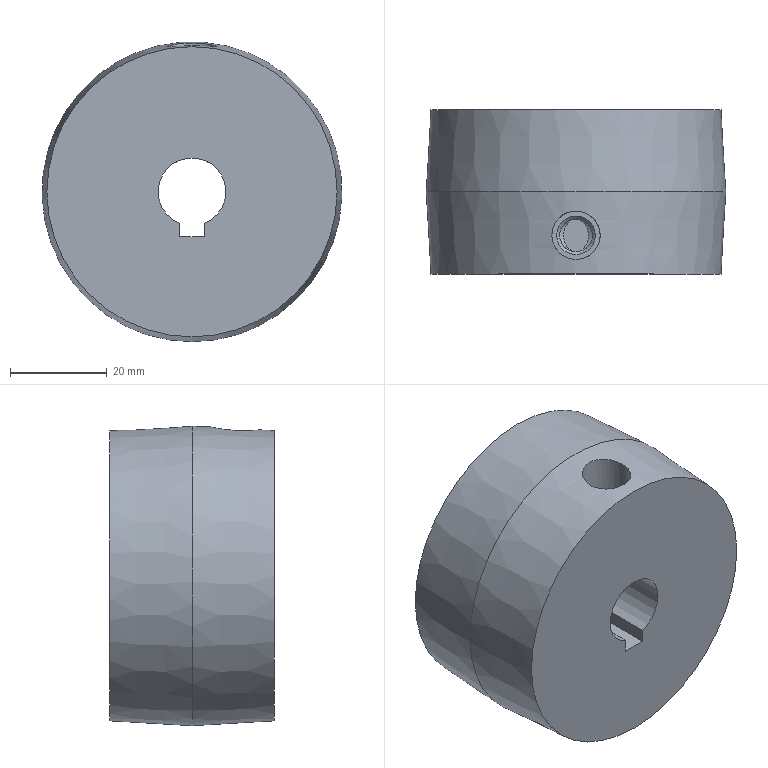Part | NX | features DATUM_CSYS 6, SKETCH 5, HOLE PACKAGE 2, SIMPLE HOLE 2, SWP104 2, EXTRUDE 1, SYMBOLIC_THREAD 1 | 1 solid | 16 faces | box 62 x 34 x 62 mm | volume 57319 mm3 | plane 7 | cone 5 | cylinder 4 | commonest cylinder face diameters 6.8 x1 10 x1 14 x1 52 x1
STEP:
#1=CARTESIAN_POINT('',(0.,0.,-30.));
#2=VERTEX_POINT('',#1);
#3=CARTESIAN_POINT('',(0.,0.,0.));
#4=DIRECTION('',(0.,-1.,0.));
#5=DIRECTION('',(0.,0.,-1.));
#6=AXIS2_PLACEMENT_3D('',#3,#4,#5);
#7=CIRCLE('',#6,30.);
#8=EDGE_CURVE('',#2,#2,#7,.T.);
#9=ORIENTED_EDGE('',*,*,#8,.F.);
#10=EDGE_LOOP('',(#9));
#11=FACE_BOUND('',#10,.T.);
#12=CARTESIAN_POINT('',(0.,17.,-31.));
#13=VERTEX_POINT('',#12);
#14=CARTESIAN_POINT('',(0.,17.,0.));
#15=DIRECTION('',(0.,-1.,0.));
#16=DIRECTION('',(0.,0.,-1.));
#17=AXIS2_PLACEMENT_3D('',#14,#15,#16);
#18=CIRCLE('',#17,31.);
#19=EDGE_CURVE('',#13,#13,#18,.T.);
#20=ORIENTED_EDGE('',*,*,#19,.T.);
#21=EDGE_LOOP('',(#20));
#22=FACE_BOUND('',#21,.T.);
#23=CARTESIAN_POINT('',(-3.572,4.502,30.053));
#24=VERTEX_POINT('',#23);
#25=CARTESIAN_POINT('',(-5.539,8.08,29.959));
#26=CARTESIAN_POINT('',(-3.962,4.118,30.028));
#27=CARTESIAN_POINT('',(-0.0481,2.459,30.249));
#28=CARTESIAN_POINT('',(3.888,4.047,30.035));
#29=CARTESIAN_POINT('',(5.541,7.972,29.952));
#30=CARTESIAN_POINT('',(3.949,11.879,30.491));
#31=CARTESIAN_POINT('',(0.05764,13.542,30.898));
#32=CARTESIAN_POINT('',(-3.879,11.952,30.507));
#33=CARTESIAN_POINT('',(-5.539,8.08,29.959));
#34=CARTESIAN_POINT('',(-3.962,4.118,30.028));
#35=CARTESIAN_POINT('',(-0.0481,2.459,30.249));
#36=B_SPLINE_CURVE_WITH_KNOTS('',3,(#25,#26,#27,#28,#29,#30,#31,#32,#33,#34,#35),.UNSPECIFIED.,.T.,.F.,(1,1,1,1,1,1,1,1,1,1,1,1,1,1,1),(-0.01175,-0.007835,-0.003918,0.,0.003918,0.007835,0.01175,0.01567,0.01959,0.02351,0.02742,0.03134,0.03526,0.03918,0.04309),.UNSPECIFIED.);
#37=EDGE_CURVE('',#24,#24,#36,.T.);
#38=ORIENTED_EDGE('',*,*,#37,.F.);
#39=EDGE_LOOP('',(#38));
#40=FACE_BOUND('',#39,.T.);
#41=CARTESIAN_POINT('',(0.,17.,0.));
#42=DIRECTION('',(0.,1.,0.));
#43=DIRECTION('',(0.,0.,1.));
#44=AXIS2_PLACEMENT_3D('',#41,#42,#43);
#45=CONICAL_SURFACE('',#44,31.,0.05876);
#46=ADVANCED_FACE('',(#11,#22,#40),#45,.T.);
#47=CARTESIAN_POINT('',(0.,16.,-26.));
#48=VERTEX_POINT('',#47);
#49=CARTESIAN_POINT('',(0.,16.,0.));
#50=DIRECTION('',(0.,-1.,0.));
#51=DIRECTION('',(0.,0.,-1.));
#52=AXIS2_PLACEMENT_3D('',#49,#50,#51);
#53=CIRCLE('',#52,26.);
#54=EDGE_CURVE('',#48,#48,#53,.F.);
#55=ORIENTED_EDGE('',*,*,#54,.T.);
#56=EDGE_LOOP('',(#55));
#57=FACE_BOUND('',#56,.T.);
#58=CARTESIAN_POINT('',(2.5,16.,-9.3));
#59=VERTEX_POINT('',#58);
#60=CARTESIAN_POINT('',(-2.5,16.,-9.3));
#61=VERTEX_POINT('',#60);
#62=CARTESIAN_POINT('',(-2.5,16.,-9.3));
#63=DIRECTION('',(-1.,0.,0.));
#64=VECTOR('',#63,1000.);
#65=LINE('',#62,#64);
#66=EDGE_CURVE('',#59,#61,#65,.T.);
#67=ORIENTED_EDGE('',*,*,#66,.F.);
#68=CARTESIAN_POINT('',(2.5,16.,-6.538));
#69=VERTEX_POINT('',#68);
#70=CARTESIAN_POINT('',(2.5,16.,-9.3));
#71=DIRECTION('',(0.,0.,-1.));
#72=VECTOR('',#71,1000.);
#73=LINE('',#70,#72);
#74=EDGE_CURVE('',#69,#59,#73,.T.);
#75=ORIENTED_EDGE('',*,*,#74,.F.);
#76=CARTESIAN_POINT('',(-2.5,16.,-6.538));
#77=VERTEX_POINT('',#76);
#78=CARTESIAN_POINT('',(0.,16.,0.));
#79=DIRECTION('',(0.,-1.,0.));
#80=DIRECTION('',(0.,0.,-1.));
#81=AXIS2_PLACEMENT_3D('',#78,#79,#80);
#82=CIRCLE('',#81,7.);
#83=EDGE_CURVE('',#77,#69,#82,.F.);
#84=ORIENTED_EDGE('',*,*,#83,.F.);
#85=CARTESIAN_POINT('',(-2.5,16.,-6.538));
#86=DIRECTION('',(0.,0.,1.));
#87=VECTOR('',#86,1000.);
#88=LINE('',#85,#87);
#89=EDGE_CURVE('',#61,#77,#88,.T.);
#90=ORIENTED_EDGE('',*,*,#89,.F.);
#91=EDGE_LOOP('',(#67,#75,#84,#90));
#92=FACE_BOUND('',#91,.T.);
#93=CARTESIAN_POINT('',(0.,16.,0.));
#94=DIRECTION('',(0.,-1.,0.));
#95=DIRECTION('',(0.,0.,-1.));
#96=AXIS2_PLACEMENT_3D('',#93,#94,#95);
#97=PLANE('',#96);
#98=ADVANCED_FACE('',(#57,#92),#97,.F.);
#99=CARTESIAN_POINT('',(2.5,0.,-9.3));
#100=VERTEX_POINT('',#99);
#101=CARTESIAN_POINT('',(2.5,0.,-6.538));
#102=VERTEX_POINT('',#101);
#103=CARTESIAN_POINT('',(2.5,0.,-9.3));
#104=DIRECTION('',(0.,0.,1.));
#105=VECTOR('',#104,1000.);
#106=LINE('',#103,#105);
#107=EDGE_CURVE('',#100,#102,#106,.T.);
#108=ORIENTED_EDGE('',*,*,#107,.F.);
#109=CARTESIAN_POINT('',(-2.5,0.,-9.3));
#110=VERTEX_POINT('',#109);
#111=CARTESIAN_POINT('',(-2.5,0.,-9.3));
#112=DIRECTION('',(1.,0.,0.));
#113=VECTOR('',#112,1000.);
#114=LINE('',#111,#113);
#115=EDGE_CURVE('',#110,#100,#114,.T.);
#116=ORIENTED_EDGE('',*,*,#115,.F.);
#117=CARTESIAN_POINT('',(-2.5,0.,-6.538));
#118=VERTEX_POINT('',#117);
#119=CARTESIAN_POINT('',(-2.5,0.,-6.538));
#120=DIRECTION('',(0.,0.,-1.));
#121=VECTOR('',#120,1000.);
#122=LINE('',#119,#121);
#123=EDGE_CURVE('',#118,#110,#122,.T.);
#124=ORIENTED_EDGE('',*,*,#123,.F.);
#125=CARTESIAN_POINT('',(0.,0.,0.));
#126=DIRECTION('',(0.,-1.,0.));
#127=DIRECTION('',(1.,0.,0.));
#128=AXIS2_PLACEMENT_3D('',#125,#126,#127);
#129=CIRCLE('',#128,7.);
#130=EDGE_CURVE('',#102,#118,#129,.T.);
#131=ORIENTED_EDGE('',*,*,#130,.F.);
#132=EDGE_LOOP('',(#108,#116,#124,#131));
#133=FACE_BOUND('',#132,.T.);
#134=ORIENTED_EDGE('',*,*,#8,.T.);
#135=EDGE_LOOP('',(#134));
#136=FACE_BOUND('',#135,.T.);
#137=CARTESIAN_POINT('',(0.,0.,30.));
#138=DIRECTION('',(0.,1.,0.));
#139=DIRECTION('',(0.,0.,1.));
#140=AXIS2_PLACEMENT_3D('',#137,#138,#139);
#141=PLANE('',#140);
#142=ADVANCED_FACE('',(#133,#136),#141,.F.);
#143=CARTESIAN_POINT('',(0.,34.,-26.));
#144=VERTEX_POINT('',#143);
#145=CARTESIAN_POINT('',(0.,34.,0.));
#146=DIRECTION('',(0.,-1.,0.));
#147=DIRECTION('',(0.,0.,-1.));
#148=AXIS2_PLACEMENT_3D('',#145,#146,#147);
#149=CIRCLE('',#148,26.);
#150=EDGE_CURVE('',#144,#144,#149,.T.);
#151=ORIENTED_EDGE('',*,*,#150,.T.);
#152=EDGE_LOOP('',(#151));
#153=FACE_BOUND('',#152,.T.);
#154=CARTESIAN_POINT('',(0.,34.,-30.));
#155=VERTEX_POINT('',#154);
#156=CARTESIAN_POINT('',(0.,34.,0.));
#157=DIRECTION('',(0.,-1.,0.));
#158=DIRECTION('',(0.,0.,-1.));
#159=AXIS2_PLACEMENT_3D('',#156,#157,#158);
#160=CIRCLE('',#159,30.);
#161=EDGE_CURVE('',#155,#155,#160,.T.);
#162=ORIENTED_EDGE('',*,*,#161,.F.);
#163=EDGE_LOOP('',(#162));
#164=FACE_BOUND('',#163,.T.);
#165=CARTESIAN_POINT('',(0.,34.,0.));
#166=DIRECTION('',(0.,-1.,0.));
#167=DIRECTION('',(0.,0.,-1.));
#168=AXIS2_PLACEMENT_3D('',#165,#166,#167);
#169=PLANE('',#168);
#170=ADVANCED_FACE('',(#153,#164),#169,.F.);
#171=ORIENTED_EDGE('',*,*,#19,.F.);
#172=EDGE_LOOP('',(#171));
#173=FACE_BOUND('',#172,.T.);
#174=ORIENTED_EDGE('',*,*,#161,.T.);
#175=EDGE_LOOP('',(#174));
#176=FACE_BOUND('',#175,.T.);
#177=CARTESIAN_POINT('',(0.,34.,0.));
#178=DIRECTION('',(0.,-1.,0.));
#179=DIRECTION('',(0.,0.,-1.));
#180=AXIS2_PLACEMENT_3D('',#177,#178,#179);
#181=CONICAL_SURFACE('',#180,30.,0.05876);
#182=ADVANCED_FACE('',(#173,#176),#181,.T.);
#183=ORIENTED_EDGE('',*,*,#54,.F.);
#184=EDGE_LOOP('',(#183));
#185=FACE_BOUND('',#184,.T.);
#186=ORIENTED_EDGE('',*,*,#150,.F.);
#187=EDGE_LOOP('',(#186));
#188=FACE_BOUND('',#187,.T.);
#189=CARTESIAN_POINT('',(0.,34.,0.));
#190=DIRECTION('',(0.,-1.,0.));
#191=DIRECTION('',(0.,0.,-1.));
#192=AXIS2_PLACEMENT_3D('',#189,#190,#191);
#193=CYLINDRICAL_SURFACE('',#192,26.);
#194=ADVANCED_FACE('',(#185,#188),#193,.F.);
#195=ORIENTED_EDGE('',*,*,#66,.T.);
#196=CARTESIAN_POINT('',(-2.5,55000.,-9.3));
#197=DIRECTION('',(0.,-1.,0.));
#198=VECTOR('',#197,1000.);
#199=LINE('',#196,#198);
#200=EDGE_CURVE('',#110,#61,#199,.F.);
#201=ORIENTED_EDGE('',*,*,#200,.F.);
#202=ORIENTED_EDGE('',*,*,#115,.T.);
#203=CARTESIAN_POINT('',(2.5,55000.,-9.3));
#204=DIRECTION('',(0.,-1.,0.));
#205=VECTOR('',#204,1000.);
#206=LINE('',#203,#205);
#207=EDGE_CURVE('',#100,#59,#206,.F.);
#208=ORIENTED_EDGE('',*,*,#207,.T.);
#209=EDGE_LOOP('',(#195,#201,#202,#208));
#210=FACE_BOUND('',#209,.T.);
#211=CARTESIAN_POINT('',(-2.5,55000.,-9.3));
#212=DIRECTION('',(0.,0.,-1.));
#213=DIRECTION('',(-1.,0.,0.));
#214=AXIS2_PLACEMENT_3D('',#211,#212,#213);
#215=PLANE('',#214);
#216=ADVANCED_FACE('',(#210),#215,.F.);
#217=ORIENTED_EDGE('',*,*,#74,.T.);
#218=ORIENTED_EDGE('',*,*,#207,.F.);
#219=ORIENTED_EDGE('',*,*,#107,.T.);
#220=CARTESIAN_POINT('',(2.5,55000.,-6.538));
#221=DIRECTION('',(0.,-1.,0.));
#222=VECTOR('',#221,1000.);
#223=LINE('',#220,#222);
#224=EDGE_CURVE('',#102,#69,#223,.F.);
#225=ORIENTED_EDGE('',*,*,#224,.T.);
#226=EDGE_LOOP('',(#217,#218,#219,#225));
#227=FACE_BOUND('',#226,.T.);
#228=CARTESIAN_POINT('',(2.5,55000.,-9.3));
#229=DIRECTION('',(1.,0.,0.));
#230=DIRECTION('',(0.,0.,-1.));
#231=AXIS2_PLACEMENT_3D('',#228,#229,#230);
#232=PLANE('',#231);
#233=ADVANCED_FACE('',(#227),#232,.F.);
#234=ORIENTED_EDGE('',*,*,#89,.T.);
#235=CARTESIAN_POINT('',(-2.5,55000.,-6.538));
#236=DIRECTION('',(0.,-1.,0.));
#237=VECTOR('',#236,1000.);
#238=LINE('',#235,#237);
#239=EDGE_CURVE('',#118,#77,#238,.F.);
#240=ORIENTED_EDGE('',*,*,#239,.F.);
#241=ORIENTED_EDGE('',*,*,#123,.T.);
#242=ORIENTED_EDGE('',*,*,#200,.T.);
#243=EDGE_LOOP('',(#234,#240,#241,#242));
#244=FACE_BOUND('',#243,.T.);
#245=CARTESIAN_POINT('',(-2.5,55000.,-6.538));
#246=DIRECTION('',(-1.,0.,0.));
#247=DIRECTION('',(0.,0.,1.));
#248=AXIS2_PLACEMENT_3D('',#245,#246,#247);
#249=PLANE('',#248);
#250=ADVANCED_FACE('',(#244),#249,.F.);
#251=CARTESIAN_POINT('',(0.,11.4,7.));
#252=VERTEX_POINT('',#251);
#253=CARTESIAN_POINT('',(0.,4.6,7.));
#254=VERTEX_POINT('',#253);
#255=CARTESIAN_POINT('',(0.,11.4,7.));
#256=CARTESIAN_POINT('',(-0.7926,11.4,7.));
#257=CARTESIAN_POINT('',(-2.181,10.356,6.702));
#258=CARTESIAN_POINT('',(-2.78,7.997,6.41));
#259=CARTESIAN_POINT('',(-2.178,5.641,6.703));
#260=CARTESIAN_POINT('',(-0.7919,4.6,7.));
#261=CARTESIAN_POINT('',(0.,4.6,7.));
#262=B_SPLINE_CURVE_WITH_KNOTS('',3,(#255,#256,#257,#258,#259,#260,#261),.UNSPECIFIED.,.F.,.F.,(4,1,1,1,4),(0.01105,0.01341,0.01576,0.01812,0.02047),.UNSPECIFIED.);
#263=EDGE_CURVE('',#252,#254,#262,.T.);
#264=ORIENTED_EDGE('',*,*,#263,.T.);
#265=CARTESIAN_POINT('',(0.,4.6,7.));
#266=CARTESIAN_POINT('',(0.7926,4.6,7.));
#267=CARTESIAN_POINT('',(2.179,5.642,6.702));
#268=CARTESIAN_POINT('',(2.781,8.006,6.41));
#269=CARTESIAN_POINT('',(2.177,10.358,6.703));
#270=CARTESIAN_POINT('',(0.7934,11.4,7.));
#271=CARTESIAN_POINT('',(0.,11.4,7.));
#272=B_SPLINE_CURVE_WITH_KNOTS('',3,(#265,#266,#267,#268,#269,#270,#271),.UNSPECIFIED.,.F.,.F.,(4,1,1,1,4),(0.001624,0.003981,0.006338,0.008695,0.01105),.UNSPECIFIED.);
#273=EDGE_CURVE('',#254,#252,#272,.T.);
#274=ORIENTED_EDGE('',*,*,#273,.T.);
#275=EDGE_LOOP('',(#264,#274));
#276=FACE_BOUND('',#275,.T.);
#277=ORIENTED_EDGE('',*,*,#83,.T.);
#278=ORIENTED_EDGE('',*,*,#224,.F.);
#279=ORIENTED_EDGE('',*,*,#130,.T.);
#280=ORIENTED_EDGE('',*,*,#239,.T.);
#281=EDGE_LOOP('',(#277,#278,#279,#280));
#282=FACE_BOUND('',#281,.T.);
#283=CARTESIAN_POINT('',(0.,55000.,0.));
#284=DIRECTION('',(0.,-1.,0.));
#285=DIRECTION('',(0.,0.,-1.));
#286=AXIS2_PLACEMENT_3D('',#283,#284,#285);
#287=CYLINDRICAL_SURFACE('',#286,7.);
#288=ADVANCED_FACE('',(#276,#282),#287,.F.);
#289=CARTESIAN_POINT('',(-5.,8.,23.));
#290=VERTEX_POINT('',#289);
#291=CARTESIAN_POINT('',(0.,8.,23.));
#292=DIRECTION('',(0.,0.,-1.));
#293=DIRECTION('',(-1.,0.,0.));
#294=AXIS2_PLACEMENT_3D('',#291,#292,#293);
#295=CIRCLE('',#294,5.);
#296=EDGE_CURVE('',#290,#290,#295,.F.);
#297=ORIENTED_EDGE('',*,*,#296,.F.);
#298=EDGE_LOOP('',(#297));
#299=FACE_BOUND('',#298,.T.);
#300=ORIENTED_EDGE('',*,*,#37,.T.);
#301=EDGE_LOOP('',(#300));
#302=FACE_BOUND('',#301,.T.);
#303=CARTESIAN_POINT('',(0.,8.,40.973));
#304=DIRECTION('',(0.,0.,-1.));
#305=DIRECTION('',(-1.,0.,0.));
#306=AXIS2_PLACEMENT_3D('',#303,#304,#305);
#307=CYLINDRICAL_SURFACE('',#306,5.);
#308=ADVANCED_FACE('',(#299,#302),#307,.F.);
#309=CARTESIAN_POINT('',(4.,8.,23.));
#310=VERTEX_POINT('',#309);
#311=CARTESIAN_POINT('',(0.,8.,23.));
#312=DIRECTION('',(0.,0.,1.));
#313=DIRECTION('',(1.,0.,0.));
#314=AXIS2_PLACEMENT_3D('',#311,#312,#313);
#315=CIRCLE('',#314,4.);
#316=EDGE_CURVE('',#310,#310,#315,.T.);
#317=ORIENTED_EDGE('',*,*,#316,.F.);
#318=EDGE_LOOP('',(#317));
#319=FACE_BOUND('',#318,.T.);
#320=ORIENTED_EDGE('',*,*,#296,.T.);
#321=EDGE_LOOP('',(#320));
#322=FACE_BOUND('',#321,.T.);
#323=CARTESIAN_POINT('',(0.,4.,23.));
#324=DIRECTION('',(0.,0.,1.));
#325=DIRECTION('',(1.,0.,0.));
#326=AXIS2_PLACEMENT_3D('',#323,#324,#325);
#327=PLANE('',#326);
#328=ADVANCED_FACE('',(#319,#322),#327,.T.);
#329=CARTESIAN_POINT('',(0.,8.,7.));
#330=DIRECTION('',(0.,0.,-1.));
#331=DIRECTION('',(-1.,0.,0.));
#332=AXIS2_PLACEMENT_3D('',#329,#330,#331);
#333=CIRCLE('',#332,3.4);
#334=EDGE_CURVE('',#254,#252,#333,.F.);
#335=ORIENTED_EDGE('',*,*,#334,.T.);
#336=ORIENTED_EDGE('',*,*,#273,.F.);
#337=EDGE_LOOP('',(#335,#336));
#338=FACE_BOUND('',#337,.T.);
#339=CARTESIAN_POINT('',(0.,8.,7.));
#340=DIRECTION('',(0.,0.,1.));
#341=DIRECTION('',(1.,0.,0.));
#342=AXIS2_PLACEMENT_3D('',#339,#340,#341);
#343=CONICAL_SURFACE('',#342,3.4,1.03);
#344=ADVANCED_FACE('',(#338),#343,.F.);
#345=CARTESIAN_POINT('',(0.,8.,7.));
#346=DIRECTION('',(0.,0.,-1.));
#347=DIRECTION('',(-1.,0.,0.));
#348=AXIS2_PLACEMENT_3D('',#345,#346,#347);
#349=CIRCLE('',#348,3.4);
#350=EDGE_CURVE('',#252,#254,#349,.F.);
#351=ORIENTED_EDGE('',*,*,#350,.T.);
#352=ORIENTED_EDGE('',*,*,#263,.F.);
#353=EDGE_LOOP('',(#351,#352));
#354=FACE_BOUND('',#353,.T.);
#355=CARTESIAN_POINT('',(0.,8.,7.));
#356=DIRECTION('',(0.,0.,1.));
#357=DIRECTION('',(1.,0.,0.));
#358=AXIS2_PLACEMENT_3D('',#355,#356,#357);
#359=CONICAL_SURFACE('',#358,3.4,1.03);
#360=ADVANCED_FACE('',(#354),#359,.F.);
#361=CARTESIAN_POINT('',(3.4,8.,22.4));
#362=VERTEX_POINT('',#361);
#363=CARTESIAN_POINT('',(0.,8.,22.4));
#364=DIRECTION('',(0.,0.,1.));
#365=DIRECTION('',(1.,0.,0.));
#366=AXIS2_PLACEMENT_3D('',#363,#364,#365);
#367=CIRCLE('',#366,3.4);
#368=EDGE_CURVE('',#362,#362,#367,.T.);
#369=ORIENTED_EDGE('',*,*,#368,.T.);
#370=EDGE_LOOP('',(#369));
#371=FACE_BOUND('',#370,.T.);
#372=ORIENTED_EDGE('',*,*,#334,.F.);
#373=ORIENTED_EDGE('',*,*,#350,.F.);
#374=EDGE_LOOP('',(#372,#373));
#375=FACE_BOUND('',#374,.T.);
#376=CARTESIAN_POINT('',(0.,8.,23.));
#377=DIRECTION('',(0.,0.,-1.));
#378=DIRECTION('',(-1.,0.,0.));
#379=AXIS2_PLACEMENT_3D('',#376,#377,#378);
#380=CYLINDRICAL_SURFACE('',#379,3.4);
#381=ADVANCED_FACE('',(#371,#375),#380,.F.);
#382=ORIENTED_EDGE('',*,*,#316,.T.);
#383=EDGE_LOOP('',(#382));
#384=FACE_BOUND('',#383,.T.);
#385=ORIENTED_EDGE('',*,*,#368,.F.);
#386=EDGE_LOOP('',(#385));
#387=FACE_BOUND('',#386,.T.);
#388=CARTESIAN_POINT('',(0.,8.,19.));
#389=DIRECTION('',(0.,0.,1.));
#390=DIRECTION('',(1.,0.,0.));
#391=AXIS2_PLACEMENT_3D('',#388,#389,#390);
#392=CONICAL_SURFACE('',#391,0.,0.7854);
#393=ADVANCED_FACE('',(#384,#387),#392,.F.);
#394=CLOSED_SHELL('',(#46,#98,#142,#170,#182,#194,#216,#233,#250,#288,#308,#328,#344,#360,#381,#393));
#395=MANIFOLD_SOLID_BREP('',#394);
#396=(LENGTH_UNIT()NAMED_UNIT(*)SI_UNIT(.MILLI.,.METRE.));
#397=UNCERTAINTY_MEASURE_WITH_UNIT(LENGTH_MEASURE(0.0508),#396,'','');
#398=(NAMED_UNIT(*)PLANE_ANGLE_UNIT()SI_UNIT($,.RADIAN.));
#399=(NAMED_UNIT(*)SI_UNIT($,.STERADIAN.)SOLID_ANGLE_UNIT());
#400=(GEOMETRIC_REPRESENTATION_CONTEXT(3)GLOBAL_UNCERTAINTY_ASSIGNED_CONTEXT((#397))GLOBAL_UNIT_ASSIGNED_CONTEXT((#396,#398,#399))REPRESENTATION_CONTEXT('',''));
#401=ADVANCED_BREP_SHAPE_REPRESENTATION('',(#395),#400);